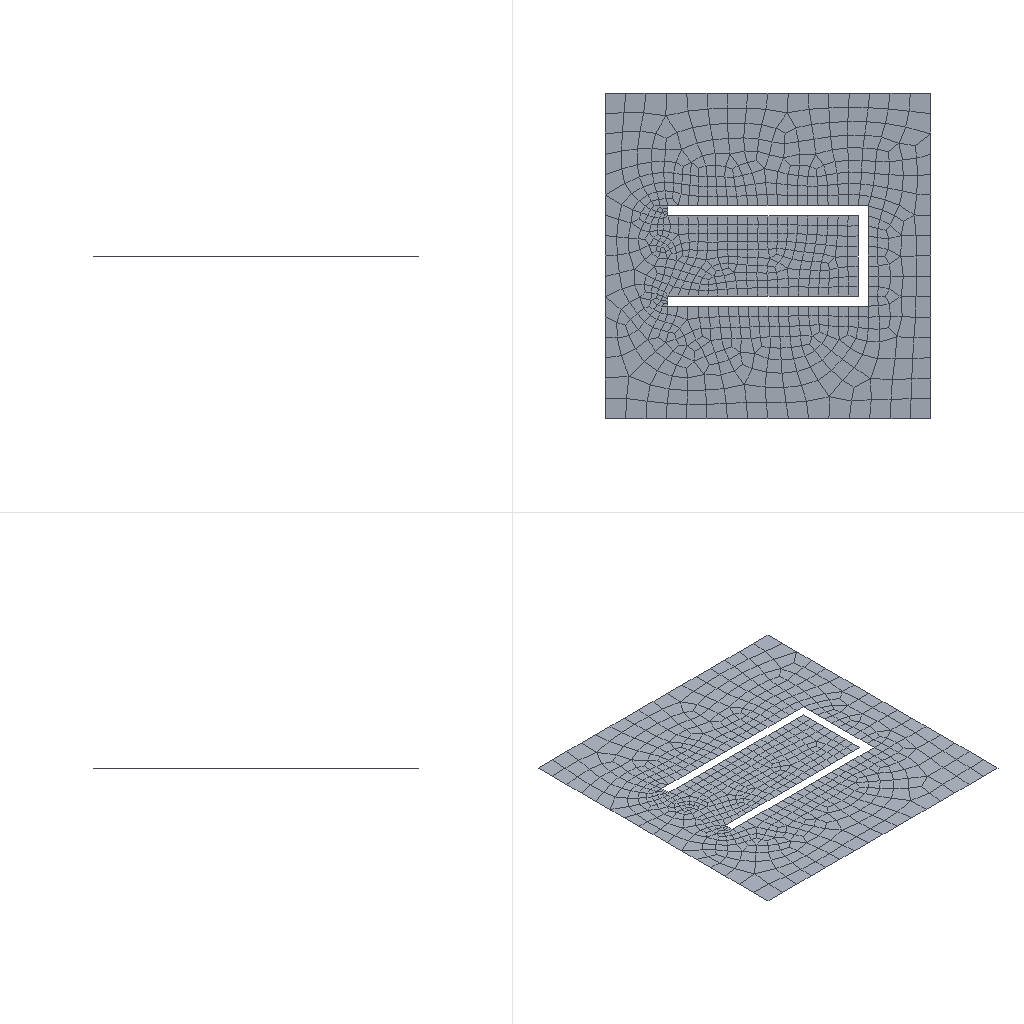Simulation study | abaqus
Set-up summary:
category,name,step,type,value,unit,region
solver,abaqus
solver,version,,,Abaqus/Explicit 2020
units,not stated in the deck,,not stated
analysis,deck,,transient,transient
load_step,Step-u,Step-u,transient
load_step,Step-1,Step-1,transient
load_step,Step-huitan,Step-huitan,transient
load_step,requested,,,3
mesh,nodes,,,1651
mesh,elements,,,1447
element_type,S4R,,shell,732
element_type,MASS,,point,3
element_type,R3D3,,rigid,6
element_type,R3D4,,rigid,703
element_type,ROTARYI,,mass,3
load,load commands in deck,,count,3
bc,support commands in deck,,count,15
material,CHUNTIE N,,in results
check,setup vs results,,match,"per instance, exact: element labels, types and connectivity; labels of the nodes the elements use; coordinates of those nodes at SINGLE_PRECISION in 4 of 4 instance(s)"
Abaqus input file, long lists of numbers shortened:
*Heading
** Job name: Job-huitan Model name: Model-1-Copy
** Generated by: Abaqus/CAE 2020
*Preprint, echo=NO, model=NO, history=NO, contact=NO
**
** PARTS
**
*Part, name=blank
*Node
      1,        1.625,       -1.625,   -2.15
      2,       -1.625,       -1.625,   -2.15
** (814 more lines like these left out)
*Element, type=S4R
  1, 700, 710, 721, 713
  2, 377, 190, 284, 454
** (730 more lines like these left out)
*Nset, nset=Set-1, generate
   1,  816,    1
*Elset, elset=Set-1, generate
   1,  732,    1
** Section: Section-1
*Shell Section, elset=Set-1, material="chuntie n"
0.3, 5
*End Part
**
*Part, name=flange
*Node
      1, -0.8958, -0.4,  -1.009
      2,          -1., -0.4,          -1.
** (394 more lines like these left out)
*Element, type=R3D4
 1,   1,  11, 118,  36
 2,  11,  12, 119, 118
** (348 more lines like these left out)
*Node
    397,  0.8738,           0.,  -1.305
*Nset, nset=flange-RefPt_, internal
397,
*Nset, nset=Set-7
 397,
*Elset, elset=flange, generate
   1,  350,    1
*Element, type=MASS, elset=Set-7_Inertia-1_MASS_
351, 397
*Mass, elset=Set-7_Inertia-1_MASS_
1.,
*Element, type=ROTARYI, elset=Set-7_Inertia-1_ROTI_
352, 397
*Rotary Inertia, elset=Set-7_Inertia-1_ROTI_
1., 1., 1., 0., 0., 0.
*End Part
**
*Part, name=pad
*Node
      1,         1.75,        -1.75,  -1.67
      2,        -1.75,        -1.75,  -1.67
** (172 more lines like these left out)
*Element, type=R3D3
1, 163,  84,  85
2, 164, 102, 103
** (2 more lines like these left out)
*Element, type=R3D4
  5,  69,  20,  21,  83
  6,  21,  22,  84,  83
** (136 more lines like these left out)
*Node
    175,        -1.75,           0.,  -1.67
*Nset, nset=pad-RefPt_, internal
175,
*Nset, nset=Set-3
 175,
*Elset, elset=pad, generate
   1,  142,    1
*Element, type=MASS, elset=Set-3_Inertia-1_MASS_
143, 175
*Mass, elset=Set-3_Inertia-1_MASS_
1.,
*Element, type=ROTARYI, elset=Set-3_Inertia-1_ROTI_
144, 175
*Rotary Inertia, elset=Set-3_Inertia-1_ROTI_
1., 1., 1., 0., 0., 0.
*End Part
**
*Part, name=post
*Node
      1,  -0.9479,  0.4,  -2.305
      2,  -0.9479, -0.4,  -2.305
** (260 more lines like these left out)
*Element, type=R3D4
1,  1, 19, 22,  4
2, 19, 20, 21, 22
** (213 more lines like these left out)
*Element, type=R3D3
28, 131, 230, 186
29, 228, 184, 133
*Node
    263,          -2.,           0.,  -2.3
*Nset, nset=post-RefPt_, internal
263,
*Nset, nset=Set-5
 263,
*Elset, elset=post, generate
   1,  217,    1
*Element, type=MASS, elset=Set-5_Inertia-1_MASS_
218, 263
*Mass, elset=Set-5_Inertia-1_MASS_
1.,
*Element, type=ROTARYI, elset=Set-5_Inertia-1_ROTI_
219, 263
*Rotary Inertia, elset=Set-5_Inertia-1_ROTI_
1., 1., 1., 0., 0., 0.
*End Part
**
**
** ASSEMBLY
**
*Assembly, name=Assembly
**
*Instance, name=post-1, part=post
*End Instance
**
*Instance, name=flange-1, part=flange
          0.,           0.,         -0.5
*End Instance
**
*Instance, name=pad-1, part=pad
          0.,           0., -0.33
*End Instance
**
*Instance, name=blank-1, part=blank
*End Instance
**
*Nset, nset=Set-1, instance=blank-1, generate
   1,  816,    1
*Elset, elset=Set-1, instance=blank-1, generate
   1,  732,    1
*Nset, nset=Set-2, instance=pad-1, generate
   1,  174,    1
*Elset, elset=Set-2, instance=pad-1, generate
   1,  142,    1
*Nset, nset=Set-7, instance=post-1
 263,
*Nset, nset=Set-8, instance=pad-1
 175,
*Nset, nset=Set-9, instance=pad-1
 175,
*Nset, nset=Set-10, instance=flange-1
 397,
*Nset, nset=Set-11, instance=blank-1
  1,  2,  3,  4, 13, 14, 15, 16, 17, 18, 19, 20, 21, 22, 23, 24
 25, 26, 27, 28, 29, 30, 31, 32, 33, 34, 35, 36, 37, 38, 39, 40
** (2 more lines like these left out)
*Elset, elset=Set-11, instance=blank-1
  25,  36,  50,  61,  63, 391, 395, 397, 410, 525, 527, 534, 539, 546, 553, 561
 569, 588, 595, 596, 597, 603, 609, 610, 611, 621, 623, 628, 632, 634, 639, 640
** (2 more lines like these left out)
*Nset, nset=Set-12, instance=blank-1
  1,  2,  3,  4, 13, 14, 15, 16, 17, 18, 19, 20, 21, 22, 23, 24
 25, 26, 27, 43, 44, 45, 46, 47, 48, 49, 50, 51, 52, 53, 54, 55
** (2 more lines like these left out)
*Elset, elset=Set-12, instance=blank-1
  25,  36,  50,  61,  63, 391, 395, 397, 410, 539, 546, 561, 588, 595, 596, 597
 603, 621, 623, 632, 634, 639, 641, 644, 645, 649, 652, 653, 663, 670, 671, 673
** (1 more lines like these left out)
*Elset, elset=_m_Surf-1_SPOS, internal, instance=pad-1, generate
   1,  142,    1
*Surface, type=ELEMENT, name=m_Surf-1
_m_Surf-1_SPOS, SPOS
*Elset, elset=_m_Surf-3_SPOS, internal, instance=flange-1, generate
   1,  350,    1
*Surface, type=ELEMENT, name=m_Surf-3
_m_Surf-3_SPOS, SPOS
*Elset, elset=_m_Surf-5_SNEG, internal, instance=post-1, generate
   1,  217,    1
*Surface, type=ELEMENT, name=m_Surf-5
_m_Surf-5_SNEG, SNEG
*Elset, elset=_s_Surf-1_SNEG, internal, instance=blank-1, generate
   1,  732,    1
*Surface, type=ELEMENT, name=s_Surf-1
_s_Surf-1_SNEG, SNEG
*Elset, elset=_s_Surf-3_SNEG, internal, instance=blank-1, generate
   1,  732,    1
*Surface, type=ELEMENT, name=s_Surf-3
_s_Surf-3_SNEG, SNEG
*Elset, elset=_s_Surf-5_SPOS, internal, instance=blank-1, generate
   1,  732,    1
*Surface, type=ELEMENT, name=s_Surf-5
_s_Surf-5_SPOS, SPOS
*Rigid Body, ref node=post-1.post-RefPt_, elset=post-1.post
*Rigid Body, ref node=flange-1.flange-RefPt_, elset=flange-1.flange
*Rigid Body, ref node=pad-1.pad-RefPt_, elset=pad-1.pad
*End Assembly
**
** MATERIALS
**
*Material, name="chuntie n"
*Density
 7.875e-09,
*Elastic
80650., 0.291
*Plastic
   98.45,   0.
 207.085, 0.02
 222.526, 0.04
 232.557, 0.06
 240.162, 0.08
 246.357,  0.1
 251.619, 0.12
 256.214, 0.14
 260.305, 0.16
  267.38,  0.2
 281.038,  0.3
 291.392,  0.4
 299.826,  0.5
  306.99,  0.6
**
** INTERACTION PROPERTIES
**
*Surface Interaction, name=IntProp-1
*Friction
 0.2,
*Surface Behavior, pressure-overclosure=HARD
**
** BOUNDARY CONDITIONS
**
** Name: BC-1 Type: 对称/反对称/完全固定
*Boundary
Set-7, ENCASTRE
** ----------------------------------------------------------------
**
** STEP: Step-u
**
*Step, name=Step-u, nlgeom=YES
*Dynamic, Explicit
, 0.001
*Bulk Viscosity
0.06, 1.2
**
** BOUNDARY CONDITIONS
**
** Name: [REDACTED] : Velocity/Angular velocity
*Boundary, type=VELOCITY
Set-9, 1, 1
Set-9, 2, 2
Set-9, 3, 3, -149.
Set-9, 4, 4
Set-9, 5, 5
Set-9, 6, 6
**
** OUTPUT REQUESTS
**
*Restart, write, number interval=1, time marks=NO
**
** FIELD OUTPUT: F-Output-1
**
*Output, field, number interval=50
*Node Output
A, RF, U, V
*Element Output, directions=YES
E, EVF, LE, MISES, PE, PEEQ, PEEQVAVG, PEVAVG, S, SSAVG, SVAVG
*Contact Output
CSTRESS,
*Output, history, frequency=0
*End Step
** ----------------------------------------------------------------
**
** STEP: Step-1
**
*Step, name=Step-1, nlgeom=YES
*Dynamic, Explicit
, 0.001
*Bulk Viscosity
0.06, 1.2
**
** BOUNDARY CONDITIONS
**
** Name: BC-3 Type: 速度/角速度
*Boundary, type=VELOCITY
Set-10, 1, 1
Set-10, 2, 2
Set-10, 3, 3, -800.
Set-10, 4, 4
Set-10, 5, 5
Set-10, 6, 6
** Name: [REDACTED] : Velocity/Angular velocity
*Boundary, type=VELOCITY
Set-9, 3, 3
**
** INTERACTIONS
**
** Interaction: Int-1
*Contact, op=NEW
*Contact Inclusions, ALL EXTERIOR
*Contact Property Assignment
 ,  , IntProp-1
**
** OUTPUT REQUESTS
**
*Restart, write, number interval=1, time marks=NO
**
** FIELD OUTPUT: F-Output-1
**
*Output, field, number interval=50
*Node Output
A, RF, U, V
*Element Output, directions=YES
E, EVF, LE, MISES, PE, PEEQ, PEEQVAVG, PEVAVG, S, SSAVG, SVAVG
*Contact Output
CSTRESS,
**
** HISTORY OUTPUT: H-Output-1
**
*Output, history, variable=PRESELECT
*End Step
** ----------------------------------------------------------------
**
** STEP: Step-huitan
**
*Step, name=Step-huitan, nlgeom=YES
*Dynamic, Explicit
, 0.01
*Bulk Viscosity
0.06, 1.2
**
** BOUNDARY CONDITIONS
**
** Name: BC-3 Type: 速度/角速度
*Boundary, type=VELOCITY
Set-10, 3, 3, 80.
**
** OUTPUT REQUESTS
**
*Restart, write, number interval=1, time marks=NO
**
** FIELD OUTPUT: F-Output-1
**
*Output, field, number interval=50
*Node Output
A, RF, U, V
*Element Output, directions=YES
E, EVF, LE, MISES, PE, PEEQ, PEEQVAVG, PEVAVG, S, SSAVG, SVAVG
*Contact Output
CSTRESS,
**
** HISTORY OUTPUT: H-Output-1
**
*Output, history, variable=PRESELECT
*End Step
Results summary:
result,step,Step-u,completed,increments=160166 time=0.001/0.001
result,step,Step-1,completed,increments=157902 time=0.001/0.001
result,step,Step-huitan,completed,increments=1556164 time=0.01/0.01
result,analysis,,,transient
result,last_loadstep,,,3
result,primary field,,,"U, UR"
result,reaction total,,FX,0.0,model units
result,reaction total,,FY,0.0,model units
result,reaction total,,FZ,0.0,model units